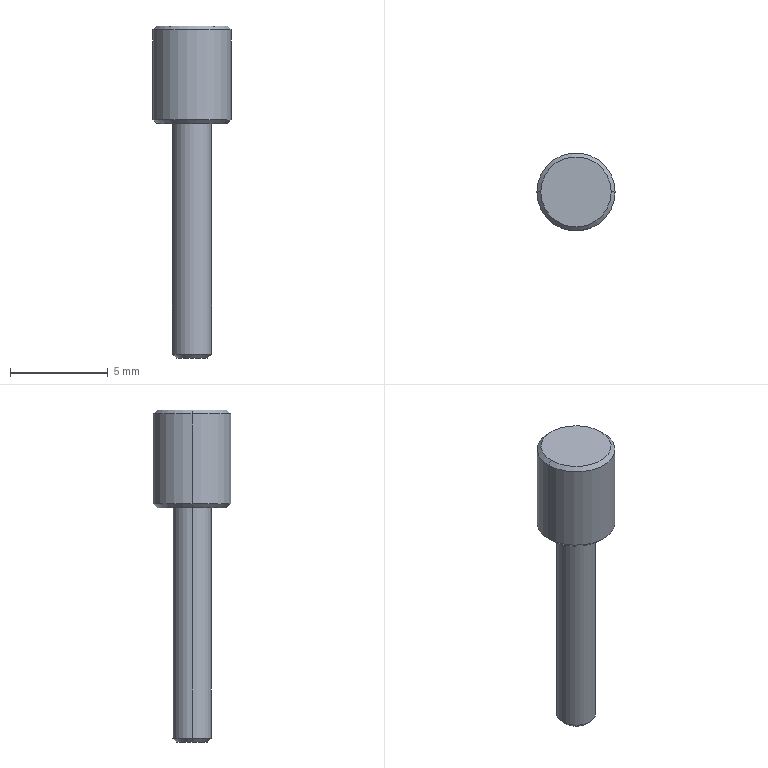Part | SolidWorks | features Chamfer 1, Extrusion 1, ICE 1 | 1 solid | 13 faces | box 4 x 4 x 17 mm | volume 99.928 mm3 | cone 6 | cylinder 4 | plane 3 | commonest cylinder face diameters 2 x2 4 x2
STEP:
#1=CARTESIAN_POINT('',(-0.8,0.,-8.5));
#2=VERTEX_POINT('',#1);
#3=CARTESIAN_POINT('',(0.8,0.,-8.5));
#4=VERTEX_POINT('',#3);
#5=CARTESIAN_POINT('',(0.,0.,-8.5));
#6=DIRECTION('',(0.,0.,-1.));
#7=DIRECTION('',(1.,0.,0.));
#8=AXIS2_PLACEMENT_3D('',#5,#6,#7);
#9=CIRCLE('',#8,0.8);
#10=EDGE_CURVE('',#2,#4,#9,.T.);
#11=ORIENTED_EDGE('',*,*,#10,.F.);
#12=CARTESIAN_POINT('',(-1.,0.,-8.3));
#13=VERTEX_POINT('',#12);
#14=CARTESIAN_POINT('',(-1.,0.,-8.3));
#15=DIRECTION('',(-0.7071,0.,0.7071));
#16=VECTOR('',#15,1000.);
#17=LINE('',#14,#16);
#18=EDGE_CURVE('',#2,#13,#17,.T.);
#19=ORIENTED_EDGE('',*,*,#18,.T.);
#20=CARTESIAN_POINT('',(1.,0.,-8.3));
#21=VERTEX_POINT('',#20);
#22=CARTESIAN_POINT('',(0.,0.,-8.3));
#23=DIRECTION('',(0.,0.,1.));
#24=DIRECTION('',(1.,0.,0.));
#25=AXIS2_PLACEMENT_3D('',#22,#23,#24);
#26=CIRCLE('',#25,1.);
#27=EDGE_CURVE('',#21,#13,#26,.T.);
#28=ORIENTED_EDGE('',*,*,#27,.F.);
#29=CARTESIAN_POINT('',(1.,0.,-8.3));
#30=DIRECTION('',(0.7071,0.,0.7071));
#31=VECTOR('',#30,1000.);
#32=LINE('',#29,#31);
#33=EDGE_CURVE('',#4,#21,#32,.T.);
#34=ORIENTED_EDGE('',*,*,#33,.F.);
#35=EDGE_LOOP('',(#11,#19,#28,#34));
#36=FACE_OUTER_BOUND('',#35,.T.);
#37=CARTESIAN_POINT('',(0.,0.,-8.3));
#38=DIRECTION('',(0.,0.,1.));
#39=DIRECTION('',(1.,0.,0.));
#40=AXIS2_PLACEMENT_3D('',#37,#38,#39);
#41=CONICAL_SURFACE('',#40,1.,0.7854);
#42=ADVANCED_FACE('',(#36),#41,.T.);
#43=CARTESIAN_POINT('',(1.8,0.,8.5));
#44=VERTEX_POINT('',#43);
#45=CARTESIAN_POINT('',(-1.8,0.,8.5));
#46=VERTEX_POINT('',#45);
#47=CARTESIAN_POINT('',(0.,0.,8.5));
#48=DIRECTION('',(0.,0.,1.));
#49=DIRECTION('',(1.,0.,0.));
#50=AXIS2_PLACEMENT_3D('',#47,#48,#49);
#51=CIRCLE('',#50,1.8);
#52=EDGE_CURVE('',#44,#46,#51,.T.);
#53=ORIENTED_EDGE('',*,*,#52,.F.);
#54=CARTESIAN_POINT('',(2.,0.,8.3));
#55=VERTEX_POINT('',#54);
#56=CARTESIAN_POINT('',(1.8,0.,8.5));
#57=DIRECTION('',(0.7071,0.,-0.7071));
#58=VECTOR('',#57,1000.);
#59=LINE('',#56,#58);
#60=EDGE_CURVE('',#44,#55,#59,.T.);
#61=ORIENTED_EDGE('',*,*,#60,.T.);
#62=CARTESIAN_POINT('',(-2.,0.,8.3));
#63=VERTEX_POINT('',#62);
#64=CARTESIAN_POINT('',(0.,0.,8.3));
#65=DIRECTION('',(0.,0.,-1.));
#66=DIRECTION('',(1.,0.,0.));
#67=AXIS2_PLACEMENT_3D('',#64,#65,#66);
#68=CIRCLE('',#67,2.);
#69=EDGE_CURVE('',#63,#55,#68,.T.);
#70=ORIENTED_EDGE('',*,*,#69,.F.);
#71=CARTESIAN_POINT('',(-1.8,0.,8.5));
#72=DIRECTION('',(-0.7071,0.,-0.7071));
#73=VECTOR('',#72,1000.);
#74=LINE('',#71,#73);
#75=EDGE_CURVE('',#46,#63,#74,.T.);
#76=ORIENTED_EDGE('',*,*,#75,.F.);
#77=EDGE_LOOP('',(#53,#61,#70,#76));
#78=FACE_OUTER_BOUND('',#77,.T.);
#79=CARTESIAN_POINT('',(0.,0.,8.5));
#80=DIRECTION('',(0.,0.,-1.));
#81=DIRECTION('',(-1.,0.,0.));
#82=AXIS2_PLACEMENT_3D('',#79,#80,#81);
#83=CONICAL_SURFACE('',#82,1.8,0.7854);
#84=ADVANCED_FACE('',(#78),#83,.T.);
#85=CARTESIAN_POINT('',(-1.8,0.,3.5));
#86=VERTEX_POINT('',#85);
#87=CARTESIAN_POINT('',(1.8,0.,3.5));
#88=VERTEX_POINT('',#87);
#89=CARTESIAN_POINT('',(0.,0.,3.5));
#90=DIRECTION('',(0.,0.,-1.));
#91=DIRECTION('',(1.,0.,0.));
#92=AXIS2_PLACEMENT_3D('',#89,#90,#91);
#93=CIRCLE('',#92,1.8);
#94=EDGE_CURVE('',#86,#88,#93,.T.);
#95=ORIENTED_EDGE('',*,*,#94,.F.);
#96=CARTESIAN_POINT('',(-2.,0.,3.7));
#97=VERTEX_POINT('',#96);
#98=CARTESIAN_POINT('',(-2.,0.,3.7));
#99=DIRECTION('',(-0.7071,0.,0.7071));
#100=VECTOR('',#99,1000.);
#101=LINE('',#98,#100);
#102=EDGE_CURVE('',#86,#97,#101,.T.);
#103=ORIENTED_EDGE('',*,*,#102,.T.);
#104=CARTESIAN_POINT('',(2.,0.,3.7));
#105=VERTEX_POINT('',#104);
#106=CARTESIAN_POINT('',(0.,0.,3.7));
#107=DIRECTION('',(0.,0.,1.));
#108=DIRECTION('',(1.,0.,0.));
#109=AXIS2_PLACEMENT_3D('',#106,#107,#108);
#110=CIRCLE('',#109,2.);
#111=EDGE_CURVE('',#105,#97,#110,.T.);
#112=ORIENTED_EDGE('',*,*,#111,.F.);
#113=CARTESIAN_POINT('',(2.,0.,3.7));
#114=DIRECTION('',(0.7071,0.,0.7071));
#115=VECTOR('',#114,1000.);
#116=LINE('',#113,#115);
#117=EDGE_CURVE('',#88,#105,#116,.T.);
#118=ORIENTED_EDGE('',*,*,#117,.F.);
#119=EDGE_LOOP('',(#95,#103,#112,#118));
#120=FACE_OUTER_BOUND('',#119,.T.);
#121=CARTESIAN_POINT('',(0.,0.,3.7));
#122=DIRECTION('',(0.,0.,1.));
#123=DIRECTION('',(1.,0.,0.));
#124=AXIS2_PLACEMENT_3D('',#121,#122,#123);
#125=CONICAL_SURFACE('',#124,2.,0.7854);
#126=ADVANCED_FACE('',(#120),#125,.T.);
#127=ORIENTED_EDGE('',*,*,#111,.T.);
#128=CARTESIAN_POINT('',(-2.,0.,3.5));
#129=DIRECTION('',(0.,0.,1.));
#130=VECTOR('',#129,1000.);
#131=LINE('',#128,#130);
#132=EDGE_CURVE('',#97,#63,#131,.T.);
#133=ORIENTED_EDGE('',*,*,#132,.T.);
#134=ORIENTED_EDGE('',*,*,#69,.T.);
#135=CARTESIAN_POINT('',(2.,0.,3.5));
#136=DIRECTION('',(0.,0.,1.));
#137=VECTOR('',#136,1000.);
#138=LINE('',#135,#137);
#139=EDGE_CURVE('',#105,#55,#138,.T.);
#140=ORIENTED_EDGE('',*,*,#139,.F.);
#141=EDGE_LOOP('',(#127,#133,#134,#140));
#142=FACE_OUTER_BOUND('',#141,.T.);
#143=CARTESIAN_POINT('',(0.,0.,3.5));
#144=DIRECTION('',(0.,0.,1.));
#145=DIRECTION('',(1.,0.,0.));
#146=AXIS2_PLACEMENT_3D('',#143,#144,#145);
#147=CYLINDRICAL_SURFACE('',#146,2.);
#148=ADVANCED_FACE('',(#142),#147,.T.);
#149=CARTESIAN_POINT('',(1.,0.,3.5));
#150=VERTEX_POINT('',#149);
#151=CARTESIAN_POINT('',(-1.,0.,3.5));
#152=VERTEX_POINT('',#151);
#153=CARTESIAN_POINT('',(0.,0.,3.5));
#154=DIRECTION('',(0.,0.,1.));
#155=DIRECTION('',(1.,0.,0.));
#156=AXIS2_PLACEMENT_3D('',#153,#154,#155);
#157=CIRCLE('',#156,1.);
#158=EDGE_CURVE('',#150,#152,#157,.T.);
#159=ORIENTED_EDGE('',*,*,#158,.F.);
#160=CARTESIAN_POINT('',(1.,0.,8.5));
#161=DIRECTION('',(0.,0.,-1.));
#162=VECTOR('',#161,1000.);
#163=LINE('',#160,#162);
#164=EDGE_CURVE('',#150,#21,#163,.T.);
#165=ORIENTED_EDGE('',*,*,#164,.T.);
#166=ORIENTED_EDGE('',*,*,#27,.T.);
#167=CARTESIAN_POINT('',(-1.,0.,8.5));
#168=DIRECTION('',(0.,0.,-1.));
#169=VECTOR('',#168,1000.);
#170=LINE('',#167,#169);
#171=EDGE_CURVE('',#152,#13,#170,.T.);
#172=ORIENTED_EDGE('',*,*,#171,.F.);
#173=EDGE_LOOP('',(#159,#165,#166,#172));
#174=FACE_OUTER_BOUND('',#173,.T.);
#175=CARTESIAN_POINT('',(0.,0.,8.5));
#176=DIRECTION('',(0.,0.,-1.));
#177=DIRECTION('',(-1.,0.,0.));
#178=AXIS2_PLACEMENT_3D('',#175,#176,#177);
#179=CYLINDRICAL_SURFACE('',#178,1.);
#180=ADVANCED_FACE('',(#174),#179,.T.);
#181=ORIENTED_EDGE('',*,*,#164,.F.);
#182=CARTESIAN_POINT('',(0.,0.,3.5));
#183=DIRECTION('',(0.,0.,1.));
#184=DIRECTION('',(1.,0.,0.));
#185=AXIS2_PLACEMENT_3D('',#182,#183,#184);
#186=CIRCLE('',#185,1.);
#187=EDGE_CURVE('',#152,#150,#186,.T.);
#188=ORIENTED_EDGE('',*,*,#187,.F.);
#189=ORIENTED_EDGE('',*,*,#171,.T.);
#190=CARTESIAN_POINT('',(0.,0.,-8.3));
#191=DIRECTION('',(0.,0.,1.));
#192=DIRECTION('',(1.,0.,0.));
#193=AXIS2_PLACEMENT_3D('',#190,#191,#192);
#194=CIRCLE('',#193,1.);
#195=EDGE_CURVE('',#13,#21,#194,.T.);
#196=ORIENTED_EDGE('',*,*,#195,.T.);
#197=EDGE_LOOP('',(#181,#188,#189,#196));
#198=FACE_OUTER_BOUND('',#197,.T.);
#199=CARTESIAN_POINT('',(0.,0.,8.5));
#200=DIRECTION('',(0.,0.,-1.));
#201=DIRECTION('',(-1.,0.,0.));
#202=AXIS2_PLACEMENT_3D('',#199,#200,#201);
#203=CYLINDRICAL_SURFACE('',#202,1.);
#204=ADVANCED_FACE('',(#198),#203,.T.);
#205=CARTESIAN_POINT('',(0.,0.,-8.5));
#206=DIRECTION('',(0.,0.,-1.));
#207=DIRECTION('',(1.,0.,0.));
#208=AXIS2_PLACEMENT_3D('',#205,#206,#207);
#209=CIRCLE('',#208,0.8);
#210=EDGE_CURVE('',#4,#2,#209,.T.);
#211=ORIENTED_EDGE('',*,*,#210,.T.);
#212=ORIENTED_EDGE('',*,*,#10,.T.);
#213=EDGE_LOOP('',(#211,#212));
#214=FACE_OUTER_BOUND('',#213,.T.);
#215=CARTESIAN_POINT('',(0.,0.,-8.5));
#216=DIRECTION('',(0.,0.,1.));
#217=DIRECTION('',(1.,0.,0.));
#218=AXIS2_PLACEMENT_3D('',#215,#216,#217);
#219=PLANE('',#218);
#220=ADVANCED_FACE('',(#214),#219,.F.);
#221=CARTESIAN_POINT('',(0.,0.,3.5));
#222=DIRECTION('',(0.,0.,-1.));
#223=DIRECTION('',(1.,0.,0.));
#224=AXIS2_PLACEMENT_3D('',#221,#222,#223);
#225=CIRCLE('',#224,1.8);
#226=EDGE_CURVE('',#88,#86,#225,.T.);
#227=ORIENTED_EDGE('',*,*,#226,.T.);
#228=ORIENTED_EDGE('',*,*,#94,.T.);
#229=EDGE_LOOP('',(#227,#228));
#230=FACE_OUTER_BOUND('',#229,.T.);
#231=ORIENTED_EDGE('',*,*,#187,.T.);
#232=ORIENTED_EDGE('',*,*,#158,.T.);
#233=EDGE_LOOP('',(#231,#232));
#234=FACE_BOUND('',#233,.T.);
#235=CARTESIAN_POINT('',(0.,0.,3.5));
#236=DIRECTION('',(0.,0.,1.));
#237=DIRECTION('',(1.,0.,0.));
#238=AXIS2_PLACEMENT_3D('',#235,#236,#237);
#239=PLANE('',#238);
#240=ADVANCED_FACE('',(#230,#234),#239,.F.);
#241=ORIENTED_EDGE('',*,*,#132,.F.);
#242=CARTESIAN_POINT('',(0.,0.,3.7));
#243=DIRECTION('',(0.,0.,1.));
#244=DIRECTION('',(1.,0.,0.));
#245=AXIS2_PLACEMENT_3D('',#242,#243,#244);
#246=CIRCLE('',#245,2.);
#247=EDGE_CURVE('',#97,#105,#246,.T.);
#248=ORIENTED_EDGE('',*,*,#247,.T.);
#249=ORIENTED_EDGE('',*,*,#139,.T.);
#250=CARTESIAN_POINT('',(0.,0.,8.3));
#251=DIRECTION('',(0.,0.,-1.));
#252=DIRECTION('',(1.,0.,0.));
#253=AXIS2_PLACEMENT_3D('',#250,#251,#252);
#254=CIRCLE('',#253,2.);
#255=EDGE_CURVE('',#55,#63,#254,.T.);
#256=ORIENTED_EDGE('',*,*,#255,.T.);
#257=EDGE_LOOP('',(#241,#248,#249,#256));
#258=FACE_OUTER_BOUND('',#257,.T.);
#259=CARTESIAN_POINT('',(0.,0.,3.5));
#260=DIRECTION('',(0.,0.,1.));
#261=DIRECTION('',(1.,0.,0.));
#262=AXIS2_PLACEMENT_3D('',#259,#260,#261);
#263=CYLINDRICAL_SURFACE('',#262,2.);
#264=ADVANCED_FACE('',(#258),#263,.T.);
#265=CARTESIAN_POINT('',(0.,0.,8.5));
#266=DIRECTION('',(0.,0.,1.));
#267=DIRECTION('',(1.,0.,0.));
#268=AXIS2_PLACEMENT_3D('',#265,#266,#267);
#269=CIRCLE('',#268,1.8);
#270=EDGE_CURVE('',#46,#44,#269,.T.);
#271=ORIENTED_EDGE('',*,*,#270,.T.);
#272=ORIENTED_EDGE('',*,*,#52,.T.);
#273=EDGE_LOOP('',(#271,#272));
#274=FACE_OUTER_BOUND('',#273,.T.);
#275=CARTESIAN_POINT('',(0.,0.,8.5));
#276=DIRECTION('',(0.,0.,1.));
#277=DIRECTION('',(1.,0.,0.));
#278=AXIS2_PLACEMENT_3D('',#275,#276,#277);
#279=PLANE('',#278);
#280=ADVANCED_FACE('',(#274),#279,.T.);
#281=ORIENTED_EDGE('',*,*,#102,.F.);
#282=ORIENTED_EDGE('',*,*,#226,.F.);
#283=ORIENTED_EDGE('',*,*,#117,.T.);
#284=ORIENTED_EDGE('',*,*,#247,.F.);
#285=EDGE_LOOP('',(#281,#282,#283,#284));
#286=FACE_OUTER_BOUND('',#285,.T.);
#287=CARTESIAN_POINT('',(0.,0.,3.7));
#288=DIRECTION('',(0.,0.,1.));
#289=DIRECTION('',(1.,0.,0.));
#290=AXIS2_PLACEMENT_3D('',#287,#288,#289);
#291=CONICAL_SURFACE('',#290,2.,0.7854);
#292=ADVANCED_FACE('',(#286),#291,.T.);
#293=ORIENTED_EDGE('',*,*,#60,.F.);
#294=ORIENTED_EDGE('',*,*,#270,.F.);
#295=ORIENTED_EDGE('',*,*,#75,.T.);
#296=ORIENTED_EDGE('',*,*,#255,.F.);
#297=EDGE_LOOP('',(#293,#294,#295,#296));
#298=FACE_OUTER_BOUND('',#297,.T.);
#299=CARTESIAN_POINT('',(0.,0.,8.5));
#300=DIRECTION('',(0.,0.,-1.));
#301=DIRECTION('',(-1.,0.,0.));
#302=AXIS2_PLACEMENT_3D('',#299,#300,#301);
#303=CONICAL_SURFACE('',#302,1.8,0.7854);
#304=ADVANCED_FACE('',(#298),#303,.T.);
#305=ORIENTED_EDGE('',*,*,#18,.F.);
#306=ORIENTED_EDGE('',*,*,#210,.F.);
#307=ORIENTED_EDGE('',*,*,#33,.T.);
#308=ORIENTED_EDGE('',*,*,#195,.F.);
#309=EDGE_LOOP('',(#305,#306,#307,#308));
#310=FACE_OUTER_BOUND('',#309,.T.);
#311=CARTESIAN_POINT('',(0.,0.,-8.3));
#312=DIRECTION('',(0.,0.,1.));
#313=DIRECTION('',(1.,0.,0.));
#314=AXIS2_PLACEMENT_3D('',#311,#312,#313);
#315=CONICAL_SURFACE('',#314,1.,0.7854);
#316=ADVANCED_FACE('',(#310),#315,.T.);
#317=CLOSED_SHELL('',(#42,#84,#126,#148,#180,#204,#220,#240,#264,#280,#292,#304,#316));
#318=MANIFOLD_SOLID_BREP('',#317);
#319=CARTESIAN_POINT('',(0.,0.,0.));
#320=DIRECTION('',(0.,0.,1.));
#321=DIRECTION('',(1.,0.,0.));
#322=AXIS2_PLACEMENT_3D('',#319,#320,#321);
#323=(LENGTH_UNIT()NAMED_UNIT(*)SI_UNIT(.MILLI.,.METRE.));
#324=UNCERTAINTY_MEASURE_WITH_UNIT(LENGTH_MEASURE(0.00001),#323,'','');
#325=(NAMED_UNIT(*)PLANE_ANGLE_UNIT()SI_UNIT($,.RADIAN.));
#326=(NAMED_UNIT(*)SI_UNIT($,.STERADIAN.)SOLID_ANGLE_UNIT());
#327=(GEOMETRIC_REPRESENTATION_CONTEXT(3)GLOBAL_UNCERTAINTY_ASSIGNED_CONTEXT((#324))GLOBAL_UNIT_ASSIGNED_CONTEXT((#323,#325,#326))REPRESENTATION_CONTEXT('',''));
#328=ADVANCED_BREP_SHAPE_REPRESENTATION('',(#318,#322),#327);